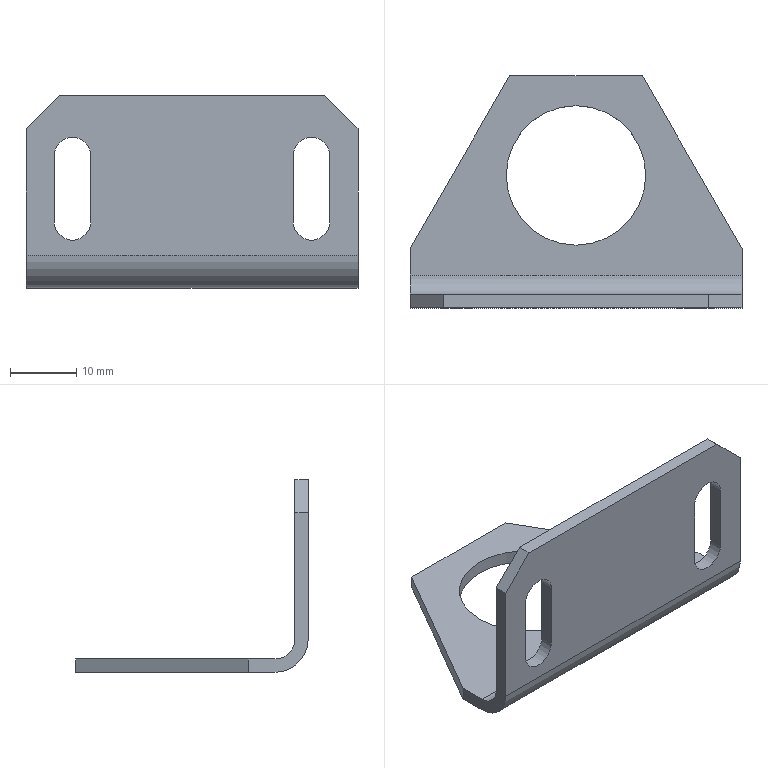Part | STEP file | CA-10-017Cylinder Mount_Default | 1 solid | 26 faces | box 50 x 35 x 29 mm | volume 4191 mm3 | plane 16 | cylinder 10 | commonest cylinder face diameters 5.5 x6 21 x2 6 x1 10 x1